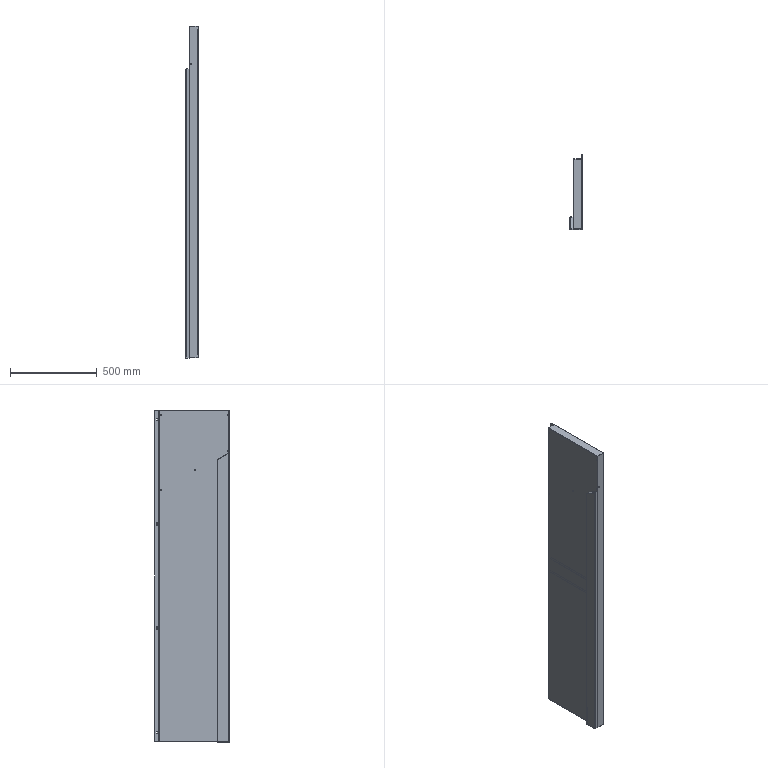Part | SolidWorks | 3 solids | 289 faces | box 70 x 430 x 1914 mm | volume 2130249 mm3 | plane 176 | cylinder 104 | spline 9 | commonest cylinder face diameters 6.4 x28 6 x14 2 x13 5 x13 7 x12 8 x8